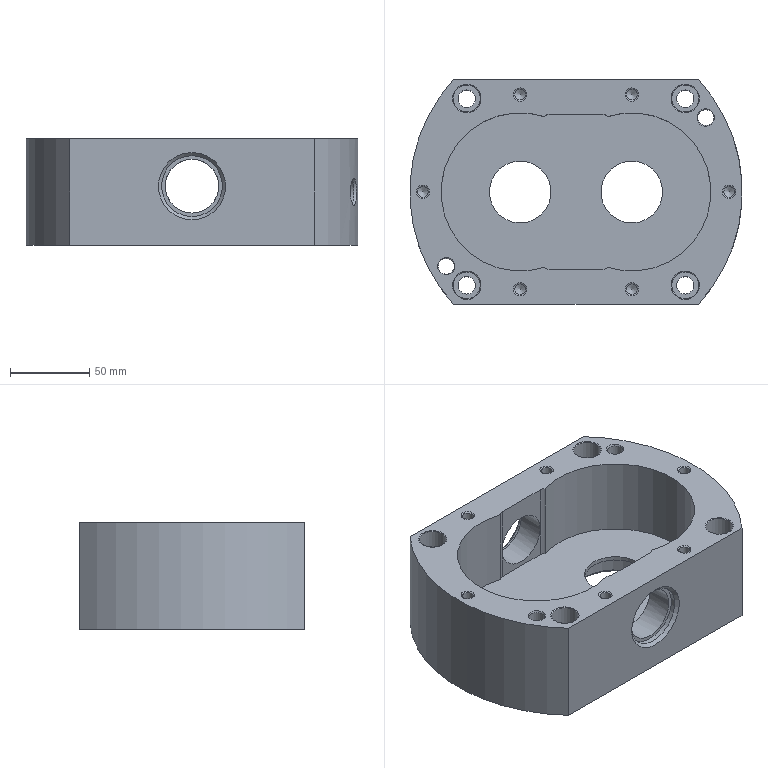NC program | NX | posted with a generic post | part box 210 x 142 x 67.4 mm
Lines 5618 to 6488 of 83330:
(ZLEVEL_PROFILE_COPY , TOOL : D6)
N11186 T06 M6
N11188 G54
N11190 G17 G0 G90 X-53.8 Y-59.497 B0. C0. S5000 M3
N11192 G43 Z30. H6
N11194 Z-0.1
N11196 G94 G1 X-54.786 Y-60.324 F1000.
N11198 G3 X-55. Y-60.784 R0.6
N11200 G1 Y-62. F1600.
N11202 G3 X-54. Y-63. R1.
N11204 G1 X-52.784
N11206 G3 X-52.324 Y-62.786 R0.6
N11208 G1 X-51.497 Y-61.8
N11210 G0 X-53.8 Y-59.497 Z-0.2
N11212 G1 X-54.786 Y-60.324 F1000.
N11214 G3 X-55. Y-60.784 R0.6
N11216 G1 Y-62. F1600.
N11218 G3 X-54. Y-63. R1.
N11220 G1 X-52.784
N11222 G3 X-52.324 Y-62.786 R0.6
N11224 G1 X-51.497 Y-61.8
N11226 G0 X-53.8 Y-59.497 Z-0.3
N11228 G1 X-54.786 Y-60.324 F1000.
N11230 G3 X-55. Y-60.784 R0.6
N11232 G1 Y-62. F1600.
N11234 G3 X-54. Y-63. R1.
N11236 G1 X-52.784
N11238 G3 X-52.324 Y-62.786 R0.6
N11240 G1 X-51.497 Y-61.8
N11242 G0 X-53.8 Y-59.497 Z-0.4
N11244 G1 X-54.786 Y-60.324 F1000.
N11246 G3 X-55. Y-60.784 R0.6
N11248 G1 Y-62. F1600.
N11250 G3 X-54. Y-63. R1.
N11252 G1 X-52.784
N11254 G3 X-52.324 Y-62.786 R0.6
N11256 G1 X-51.497 Y-61.8
N11258 G0 X-53.8 Y-59.497 Z-0.5
N11260 G1 X-54.786 Y-60.324 F1000.
N11262 G3 X-55. Y-60.784 R0.6
N11264 G1 Y-62. F1600.
N11266 G3 X-54. Y-63. R1.
N11268 G1 X-52.784
N11270 G3 X-52.324 Y-62.786 R0.6
N11272 G1 X-51.497 Y-61.8
N11274 G0 X-53.8 Y-59.497 Z-0.6
N11276 G1 X-54.786 Y-60.324 F1000.
N11278 G3 X-55. Y-60.784 R0.6
N11280 G1 Y-62. F1600.
N11282 G3 X-54. Y-63. R1.
N11284 G1 X-52.784
N11286 G3 X-52.324 Y-62.786 R0.6
N11288 G1 X-51.497 Y-61.8
N11290 G0 X-53.8 Y-59.497 Z-0.7
N11292 G1 X-54.786 Y-60.324 F1000.
N11294 G3 X-55. Y-60.784 R0.6
N11296 G1 Y-62. F1600.
N11298 G3 X-54. Y-63. R1.
N11300 G1 X-52.784
N11302 G3 X-52.324 Y-62.786 R0.6
N11304 G1 X-51.497 Y-61.8
N11306 G0 X-53.8 Y-59.497 Z-0.8
N11308 G1 X-54.786 Y-60.324 F1000.
N11310 G3 X-55. Y-60.784 R0.6
N11312 G1 Y-62. F1600.
N11314 G3 X-54. Y-63. R1.
N11316 G1 X-52.784
N11318 G3 X-52.324 Y-62.786 R0.6
N11320 G1 X-51.497 Y-61.8
N11322 G0 X-53.8 Y-59.497 Z-0.9
N11324 G1 X-54.786 Y-60.324 F1000.
N11326 G3 X-55. Y-60.784 R0.6
N11328 G1 Y-62. F1600.
N11330 G3 X-54. Y-63. R1.
N11332 G1 X-52.784
N11334 G3 X-52.324 Y-62.786 R0.6
N11336 G1 X-51.497 Y-61.8
N11338 G0 X-53.8 Y-59.497 Z-1.
N11340 G1 X-54.786 Y-60.324 F1000.
N11342 G3 X-55. Y-60.784 R0.6
N11344 G1 Y-62. F1600.
N11346 G3 X-54. Y-63. R1.
N11348 G1 X-52.784
N11350 G3 X-52.324 Y-62.786 R0.6
N11352 G1 X-51.497 Y-61.8
N11354 G0 X-53.8 Y-59.497 Z-1.1
N11356 G1 X-54.786 Y-60.324 F1000.
N11358 G3 X-55. Y-60.784 R0.6
N11360 G1 Y-62. F1600.
N11362 G3 X-54. Y-63. R1.
N11364 G1 X-52.784
N11366 G3 X-52.324 Y-62.786 R0.6
N11368 G1 X-51.497 Y-61.8
N11370 G0 X-53.8 Y-59.497 Z-1.2
N11372 G1 X-54.786 Y-60.324 F1000.
N11374 G3 X-55. Y-60.784 R0.6
N11376 G1 Y-62. F1600.
N11378 G3 X-54. Y-63. R1.
N11380 G1 X-52.784
N11382 G3 X-52.324 Y-62.786 R0.6
N11384 G1 X-51.497 Y-61.8
N11386 G0 X-53.8 Y-59.497 Z-1.3
N11388 G1 X-54.786 Y-60.324 F1000.
N11390 G3 X-55. Y-60.784 R0.6
N11392 G1 Y-62. F1600.
N11394 G3 X-54. Y-63. R1.
N11396 G1 X-52.784
N11398 G3 X-52.324 Y-62.786 R0.6
N11400 G1 X-51.497 Y-61.8
N11402 G0 X-53.8 Y-59.497 Z-1.4
N11404 G1 X-54.786 Y-60.324 F1000.
N11406 G3 X-55. Y-60.784 R0.6
N11408 G1 Y-62. F1600.
N11410 G3 X-54. Y-63. R1.
N11412 G1 X-52.784
N11414 G3 X-52.324 Y-62.786 R0.6
N11416 G1 X-51.497 Y-61.8
N11418 G0 X-53.8 Y-59.497 Z-1.5
N11420 G1 X-54.786 Y-60.324 F1000.
N11422 G3 X-55. Y-60.784 R0.6
N11424 G1 Y-62. F1600.
N11426 G3 X-54. Y-63. R1.
N11428 G1 X-52.784
N11430 G3 X-52.324 Y-62.786 R0.6
N11432 G1 X-51.497 Y-61.8
N11434 G0 X-53.8 Y-59.497 Z-1.6
N11436 G1 X-54.786 Y-60.324 F1000.
N11438 G3 X-55. Y-60.784 R0.6
N11440 G1 Y-62. F1600.
N11442 G3 X-54. Y-63. R1.
N11444 G1 X-52.784
N11446 G3 X-52.324 Y-62.786 R0.6
N11448 G1 X-51.497 Y-61.8
N11450 G0 X-53.8 Y-59.497 Z-1.7
N11452 G1 X-54.786 Y-60.324 F1000.
N11454 G3 X-55. Y-60.784 R0.6
N11456 G1 Y-62. F1600.
N11458 G3 X-54. Y-63. R1.
N11460 G1 X-52.784
N11462 G3 X-52.324 Y-62.786 R0.6
N11464 G1 X-51.497 Y-61.8
N11466 G0 X-53.8 Y-59.497 Z-1.8
N11468 G1 X-54.786 Y-60.324 F1000.
N11470 G3 X-55. Y-60.784 R0.6
N11472 G1 Y-62. F1600.
N11474 G3 X-54. Y-63. R1.
N11476 G1 X-52.784
N11478 G3 X-52.324 Y-62.786 R0.6
N11480 G1 X-51.497 Y-61.8
N11482 G0 X-53.8 Y-59.497 Z-1.9
N11484 G1 X-54.786 Y-60.324 F1000.
N11486 G3 X-55. Y-60.784 R0.6
N11488 G1 Y-62. F1600.
N11490 G3 X-54. Y-63. R1.
N11492 G1 X-52.784
N11494 G3 X-52.324 Y-62.786 R0.6
N11496 G1 X-51.497 Y-61.8
N11498 G0 X-53.8 Y-59.497 Z-2.
N11500 G1 X-54.786 Y-60.324 F1000.
N11502 G3 X-55. Y-60.784 R0.6
N11504 G1 Y-62. F1600.
N11506 G3 X-54. Y-63. R1.
N11508 G1 X-52.784
N11510 G3 X-52.324 Y-62.786 R0.6
N11512 G1 X-51.497 Y-61.8
N11514 G0 X-53.8 Y-59.497 Z-2.1
N11516 G1 X-54.786 Y-60.324 F1000.
N11518 G3 X-55. Y-60.784 R0.6
N11520 G1 Y-62. F1600.
N11522 G3 X-54. Y-63. R1.
N11524 G1 X-52.784
N11526 G3 X-52.324 Y-62.786 R0.6
N11528 G1 X-51.497 Y-61.8
N11530 G0 X-53.8 Y-59.497 Z-2.2
N11532 G1 X-54.786 Y-60.324 F1000.
N11534 G3 X-55. Y-60.784 R0.6
N11536 G1 Y-62. F1600.
N11538 G3 X-54. Y-63. R1.
N11540 G1 X-52.784
N11542 G3 X-52.324 Y-62.786 R0.6
N11544 G1 X-51.497 Y-61.8
N11546 G0 X-53.8 Y-59.497 Z-2.3
N11548 G1 X-54.786 Y-60.324 F1000.
N11550 G3 X-55. Y-60.784 R0.6
N11552 G1 Y-62. F1600.
N11554 G3 X-54. Y-63. R1.
N11556 G1 X-52.784
N11558 G3 X-52.324 Y-62.786 R0.6
N11560 G1 X-51.497 Y-61.8
N11562 G0 X-53.8 Y-59.497 Z-2.4
N11564 G1 X-54.786 Y-60.324 F1000.
N11566 G3 X-55. Y-60.784 R0.6
N11568 G1 Y-62. F1600.
N11570 G3 X-54. Y-63. R1.
N11572 G1 X-52.784
N11574 G3 X-52.324 Y-62.786 R0.6
N11576 G1 X-51.497 Y-61.8
N11578 G0 X-53.8 Y-59.497 Z-2.5
N11580 G1 X-54.786 Y-60.324 F1000.
N11582 G3 X-55. Y-60.784 R0.6
N11584 G1 Y-62. F1600.
N11586 G3 X-54. Y-63. R1.
N11588 G1 X-52.784
N11590 G3 X-52.324 Y-62.786 R0.6
N11592 G1 X-51.497 Y-61.8
N11594 G0 X-53.8 Y-59.497 Z-2.6
N11596 G1 X-54.786 Y-60.324 F1000.
N11598 G3 X-55. Y-60.784 R0.6
N11600 G1 Y-62. F1600.
N11602 G3 X-54. Y-63. R1.
N11604 G1 X-52.784
N11606 G3 X-52.324 Y-62.786 R0.6
N11608 G1 X-51.497 Y-61.8
N11610 G0 X-53.8 Y-59.497 Z-2.7
N11612 G1 X-54.786 Y-60.324 F1000.
N11614 G3 X-55. Y-60.784 R0.6
N11616 G1 Y-62. F1600.
N11618 G3 X-54. Y-63. R1.
N11620 G1 X-52.784
N11622 G3 X-52.324 Y-62.786 R0.6
N11624 G1 X-51.497 Y-61.8
N11626 G0 X-53.8 Y-59.497 Z-2.8
N11628 G1 X-54.786 Y-60.324 F1000.
N11630 G3 X-55. Y-60.784 R0.6
N11632 G1 Y-62. F1600.
N11634 G3 X-54. Y-63. R1.
N11636 G1 X-52.784
N11638 G3 X-52.324 Y-62.786 R0.6
N11640 G1 X-51.497 Y-61.8
N11642 G0 X-53.8 Y-59.497 Z-2.9
N11644 G1 X-54.786 Y-60.324 F1000.
N11646 G3 X-55. Y-60.784 R0.6
N11648 G1 Y-62. F1600.
N11650 G3 X-54. Y-63. R1.
N11652 G1 X-52.784
N11654 G3 X-52.324 Y-62.786 R0.6
N11656 G1 X-51.497 Y-61.8
N11658 G0 X-53.8 Y-59.497 Z-3.
N11660 G1 X-54.786 Y-60.324 F1000.
N11662 G3 X-55. Y-60.784 R0.6
N11664 G1 Y-62. F1600.
N11666 G3 X-54. Y-63. R1.
N11668 G1 X-52.784
N11670 G3 X-52.324 Y-62.786 R0.6
N11672 G1 X-51.497 Y-61.8
N11674 G0 X-53.8 Y-59.497 Z-3.1
N11676 G1 X-54.786 Y-60.324 F1000.
N11678 G3 X-55. Y-60.784 R0.6
N11680 G1 Y-62. F1600.
N11682 G3 X-54. Y-63. R1.
N11684 G1 X-52.784
N11686 G3 X-52.324 Y-62.786 R0.6
N11688 G1 X-51.497 Y-61.8
N11690 G0 X-53.8 Y-59.497 Z-3.2
N11692 G1 X-54.786 Y-60.324 F1000.
N11694 G3 X-55. Y-60.784 R0.6
N11696 G1 Y-62. F1600.
N11698 G3 X-54. Y-63. R1.
N11700 G1 X-52.784
N11702 G3 X-52.324 Y-62.786 R0.6
N11704 G1 X-51.497 Y-61.8
N11706 G0 X-53.8 Y-59.497 Z-3.3
N11708 G1 X-54.786 Y-60.324 F1000.
N11710 G3 X-55. Y-60.784 R0.6
N11712 G1 Y-62. F1600.
N11714 G3 X-54. Y-63. R1.
N11716 G1 X-52.784
N11718 G3 X-52.324 Y-62.786 R0.6
N11720 G1 X-51.497 Y-61.8
N11722 G0 X-53.8 Y-59.497 Z-3.4
N11724 G1 X-54.786 Y-60.324 F1000.
N11726 G3 X-55. Y-60.784 R0.6
N11728 G1 Y-62. F1600.
N11730 G3 X-54. Y-63. R1.
N11732 G1 X-52.784
N11734 G3 X-52.324 Y-62.786 R0.6
N11736 G1 X-51.497 Y-61.8
N11738 G0 X-53.8 Y-59.497 Z-3.5
N11740 G1 X-54.786 Y-60.324 F1000.
N11742 G3 X-55. Y-60.784 R0.6
N11744 G1 Y-62. F1600.
N11746 G3 X-54. Y-63. R1.
N11748 G1 X-52.784
N11750 G3 X-52.324 Y-62.786 R0.6
N11752 G1 X-51.497 Y-61.8
N11754 G0 X-53.8 Y-59.497 Z-3.6
N11756 G1 X-54.786 Y-60.324 F1000.
N11758 G3 X-55. Y-60.784 R0.6
N11760 G1 Y-62. F1600.
N11762 G3 X-54. Y-63. R1.
N11764 G1 X-52.784
N11766 G3 X-52.324 Y-62.786 R0.6
N11768 G1 X-51.497 Y-61.8
N11770 G0 X-53.8 Y-59.497 Z-3.7
N11772 G1 X-54.786 Y-60.324 F1000.
N11774 G3 X-55. Y-60.784 R0.6
N11776 G1 Y-62. F1600.
N11778 G3 X-54. Y-63. R1.
N11780 G1 X-52.784
N11782 G3 X-52.324 Y-62.786 R0.6
N11784 G1 X-51.497 Y-61.8
N11786 G0 X-53.8 Y-59.497 Z-3.8
N11788 G1 X-54.786 Y-60.324 F1000.
N11790 G3 X-55. Y-60.784 R0.6
N11792 G1 Y-62. F1600.
N11794 G3 X-54. Y-63. R1.
N11796 G1 X-52.784
N11798 G3 X-52.324 Y-62.786 R0.6
N11800 G1 X-51.497 Y-61.8
N11802 G0 X-53.8 Y-59.497 Z-3.9
N11804 G1 X-54.786 Y-60.324 F1000.
N11806 G3 X-55. Y-60.784 R0.6
N11808 G1 Y-62. F1600.
N11810 G3 X-54. Y-63. R1.
N11812 G1 X-52.784
N11814 G3 X-52.324 Y-62.786 R0.6
N11816 G1 X-51.497 Y-61.8
N11818 G0 X-53.8 Y-59.497 Z-4.
N11820 G1 X-54.786 Y-60.324 F1000.
N11822 G3 X-55. Y-60.784 R0.6
N11824 G1 Y-62. F1600.
N11826 G3 X-54. Y-63. R1.
N11828 G1 X-52.784
N11830 G3 X-52.324 Y-62.786 R0.6
N11832 G1 X-51.497 Y-61.8
N11834 G0 X-53.8 Y-59.497 Z-4.1
N11836 G1 X-54.786 Y-60.324 F1000.
N11838 G3 X-55. Y-60.784 R0.6
N11840 G1 Y-62. F1600.
N11842 G3 X-54. Y-63. R1.
N11844 G1 X-52.784
N11846 G3 X-52.324 Y-62.786 R0.6
N11848 G1 X-51.497 Y-61.8
N11850 G0 X-53.8 Y-59.497 Z-4.2
N11852 G1 X-54.786 Y-60.324 F1000.
N11854 G3 X-55. Y-60.784 R0.6
N11856 G1 Y-62. F1600.
N11858 G3 X-54. Y-63. R1.
N11860 G1 X-52.784
N11862 G3 X-52.324 Y-62.786 R0.6
N11864 G1 X-51.497 Y-61.8
N11866 G0 X-53.8 Y-59.497 Z-4.3
N11868 G1 X-54.786 Y-60.324 F1000.
N11870 G3 X-55. Y-60.784 R0.6
N11872 G1 Y-62. F1600.
N11874 G3 X-54. Y-63. R1.
N11876 G1 X-52.784
N11878 G3 X-52.324 Y-62.786 R0.6
N11880 G1 X-51.497 Y-61.8
N11882 G0 X-53.8 Y-59.497 Z-4.4
N11884 G1 X-54.786 Y-60.324 F1000.
N11886 G3 X-55. Y-60.784 R0.6
N11888 G1 Y-62. F1600.
N11890 G3 X-54. Y-63. R1.
N11892 G1 X-52.784
N11894 G3 X-52.324 Y-62.786 R0.6
N11896 G1 X-51.497 Y-61.8
N11898 G0 X-53.8 Y-59.497 Z-4.5
N11900 G1 X-54.786 Y-60.324 F1000.
N11902 G3 X-55. Y-60.784 R0.6
N11904 G1 Y-62. F1600.
N11906 G3 X-54. Y-63. R1.
N11908 G1 X-52.784
N11910 G3 X-52.324 Y-62.786 R0.6
N11912 G1 X-51.497 Y-61.8
N11914 G0 X-53.8 Y-59.497 Z-4.6
N11916 G1 X-54.786 Y-60.324 F1000.
N11918 G3 X-55. Y-60.784 R0.6
N11920 G1 Y-62. F1600.
N11922 G3 X-54. Y-63. R1.
N11924 G1 X-52.784
N11926 G3 X-52.324 Y-62.786 R0.6
N11928 G1 X-51.497 Y-61.8
N11930 G0 X-53.8 Y-59.497 Z-4.7
N11932 G1 X-54.786 Y-60.324 F1000.
N11934 G3 X-55. Y-60.784 R0.6
N11936 G1 Y-62. F1600.
N11938 G3 X-54. Y-63. R1.
N11940 G1 X-52.784
N11942 G3 X-52.324 Y-62.786 R0.6
N11944 G1 X-51.497 Y-61.8
N11946 G0 X-53.8 Y-59.497 Z-4.8
N11948 G1 X-54.786 Y-60.324 F1000.
N11950 G3 X-55. Y-60.784 R0.6
N11952 G1 Y-62. F1600.
N11954 G3 X-54. Y-63. R1.
N11956 G1 X-52.784
N11958 G3 X-52.324 Y-62.786 R0.6
N11960 G1 X-51.497 Y-61.8
N11962 G0 X-53.8 Y-59.497 Z-4.9
N11964 G1 X-54.786 Y-60.324 F1000.
N11966 G3 X-55. Y-60.784 R0.6
N11968 G1 Y-62. F1600.
N11970 G3 X-54. Y-63. R1.
N11972 G1 X-52.784
N11974 G3 X-52.324 Y-62.786 R0.6
N11976 G1 X-51.497 Y-61.8
N11978 G0 X-53.8 Y-59.497 Z-5.
N11980 G1 X-54.786 Y-60.324 F1000.
N11982 G3 X-55. Y-60.784 R0.6
N11984 G1 Y-62. F1600.
N11986 G3 X-54. Y-63. R1.
N11988 G1 X-52.784
N11990 G3 X-52.324 Y-62.786 R0.6
N11992 G1 X-51.497 Y-61.8
N11994 G0 X-53.8 Y-59.497 Z-5.1
N11996 G1 X-54.786 Y-60.324 F1000.
N11998 G3 X-55. Y-60.784 R0.6
N12000 G1 Y-62. F1600.
N12002 G3 X-54. Y-63. R1.
N12004 G1 X-52.784
N12006 G3 X-52.324 Y-62.786 R0.6
N12008 G1 X-51.497 Y-61.8
N12010 G0 X-53.8 Y-59.497 Z-5.2
N12012 G1 X-54.786 Y-60.324 F1000.
N12014 G3 X-55. Y-60.784 R0.6
N12016 G1 Y-62. F1600.
N12018 G3 X-54. Y-63. R1.
N12020 G1 X-52.784
N12022 G3 X-52.324 Y-62.786 R0.6
N12024 G1 X-51.497 Y-61.8
N12026 G0 X-53.8 Y-59.497 Z-5.3
N12028 G1 X-54.786 Y-60.324 F1000.
N12030 G3 X-55. Y-60.784 R0.6
N12032 G1 Y-62. F1600.
N12034 G3 X-54. Y-63. R1.
N12036 G1 X-52.784
N12038 G3 X-52.324 Y-62.786 R0.6
N12040 G1 X-51.497 Y-61.8
N12042 G0 X-53.8 Y-59.497 Z-5.4
N12044 G1 X-54.786 Y-60.324 F1000.
N12046 G3 X-55. Y-60.784 R0.6
N12048 G1 Y-62. F1600.
N12050 G3 X-54. Y-63. R1.
N12052 G1 X-52.784
N12054 G3 X-52.324 Y-62.786 R0.6
N12056 G1 X-51.497 Y-61.8
N12058 G0 X-53.8 Y-59.497 Z-5.5
N12060 G1 X-54.786 Y-60.324 F1000.
N12062 G3 X-55. Y-60.784 R0.6
N12064 G1 Y-62. F1600.
N12066 G3 X-54. Y-63. R1.
N12068 G1 X-52.784
N12070 G3 X-52.324 Y-62.786 R0.6
N12072 G1 X-51.497 Y-61.8
N12074 G0 X-53.8 Y-59.497 Z-5.6
N12076 G1 X-54.786 Y-60.324 F1000.
N12078 G3 X-55. Y-60.784 R0.6
N12080 G1 Y-62. F1600.
N12082 G3 X-54. Y-63. R1.
N12084 G1 X-52.784
N12086 G3 X-52.324 Y-62.786 R0.6
N12088 G1 X-51.497 Y-61.8
N12090 G0 X-53.8 Y-59.497 Z-5.7
N12092 G1 X-54.786 Y-60.324 F1000.
N12094 G3 X-55. Y-60.784 R0.6
N12096 G1 Y-62. F1600.
N12098 G3 X-54. Y-63. R1.
N12100 G1 X-52.784
N12102 G3 X-52.324 Y-62.786 R0.6
N12104 G1 X-51.497 Y-61.8
N12106 G0 X-53.8 Y-59.497 Z-5.8
N12108 G1 X-54.786 Y-60.324 F1000.
N12110 G3 X-55. Y-60.784 R0.6
N12112 G1 Y-62. F1600.
N12114 G3 X-54. Y-63. R1.
N12116 G1 X-52.784
N12118 G3 X-52.324 Y-62.786 R0.6
N12120 G1 X-51.497 Y-61.8
N12122 G0 X-53.8 Y-59.497 Z-5.9
N12124 G1 X-54.786 Y-60.324 F1000.
N12126 G3 X-55. Y-60.784 R0.6
N12128 G1 Y-62. F1600.
N12130 G3 X-54. Y-63. R1.
N12132 G1 X-52.784
N12134 G3 X-52.324 Y-62.786 R0.6
N12136 G1 X-51.497 Y-61.8
N12138 G0 X-53.8 Y-59.497 Z-6.
N12140 G1 X-54.786 Y-60.324 F1000.
N12142 G3 X-55. Y-60.784 R0.6
N12144 G1 Y-62. F1600.
N12146 G3 X-54. Y-63. R1.
N12148 G1 X-52.784
N12150 G3 X-52.324 Y-62.786 R0.6
N12152 G1 X-51.497 Y-61.8
N12154 G0 X-53.8 Y-59.497 Z-6.1
N12156 G1 X-54.786 Y-60.324 F1000.
N12158 G3 X-55. Y-60.784 R0.6
N12160 G1 Y-62. F1600.
N12162 G3 X-54. Y-63. R1.
N12164 G1 X-52.784
N12166 G3 X-52.324 Y-62.786 R0.6
N12168 G1 X-51.497 Y-61.8
N12170 G0 X-53.8 Y-59.497 Z-6.2
N12172 G1 X-54.786 Y-60.324 F1000.
N12174 G3 X-55. Y-60.784 R0.6
N12176 G1 Y-62. F1600.
N12178 G3 X-54. Y-63. R1.
N12180 G1 X-52.784
N12182 G3 X-52.324 Y-62.786 R0.6
N12184 G1 X-51.497 Y-61.8
N12186 G0 X-53.8 Y-59.497 Z-6.3
N12188 G1 X-54.786 Y-60.324 F1000.
N12190 G3 X-55. Y-60.784 R0.6
N12192 G1 Y-62. F1600.
N12194 G3 X-54. Y-63. R1.
N12196 G1 X-52.784
N12198 G3 X-52.324 Y-62.786 R0.6
N12200 G1 X-51.497 Y-61.8
N12202 G0 X-53.8 Y-59.497 Z-6.4
N12204 G1 X-54.786 Y-60.324 F1000.
N12206 G3 X-55. Y-60.784 R0.6
N12208 G1 Y-62. F1600.
N12210 G3 X-54. Y-63. R1.
N12212 G1 X-52.784
N12214 G3 X-52.324 Y-62.786 R0.6
N12216 G1 X-51.497 Y-61.8
N12218 G0 X-53.8 Y-59.497 Z-6.5
N12220 G1 X-54.786 Y-60.324 F1000.
N12222 G3 X-55. Y-60.784 R0.6
N12224 G1 Y-62. F1600.
N12226 G3 X-54. Y-63. R1.
N12228 G1 X-52.784
N12230 G3 X-52.324 Y-62.786 R0.6
N12232 G1 X-51.497 Y-61.8
N12234 G0 X-53.8 Y-59.497 Z-6.6
N12236 G1 X-54.786 Y-60.324 F1000.
N12238 G3 X-55. Y-60.784 R0.6
N12240 G1 Y-62. F1600.
N12242 G3 X-54. Y-63. R1.
N12244 G1 X-52.784
N12246 G3 X-52.324 Y-62.786 R0.6
N12248 G1 X-51.497 Y-61.8
N12250 G0 X-53.8 Y-59.497 Z-6.7
N12252 G1 X-54.786 Y-60.324 F1000.
N12254 G3 X-55. Y-60.784 R0.6
N12256 G1 Y-62. F1600.
N12258 G3 X-54. Y-63. R1.
N12260 G1 X-52.784
N12262 G3 X-52.324 Y-62.786 R0.6
N12264 G1 X-51.497 Y-61.8
N12266 G0 X-53.8 Y-59.497 Z-6.8
N12268 G1 X-54.786 Y-60.324 F1000.
N12270 G3 X-55. Y-60.784 R0.6
N12272 G1 Y-62. F1600.
N12274 G3 X-54. Y-63. R1.
N12276 G1 X-52.784
N12278 G3 X-52.324 Y-62.786 R0.6
N12280 G1 X-51.497 Y-61.8
N12282 G0 X-53.8 Y-59.497 Z-6.9
N12284 G1 X-54.786 Y-60.324 F1000.
N12286 G3 X-55. Y-60.784 R0.6
N12288 G1 Y-62. F1600.
N12290 G3 X-54. Y-63. R1.
N12292 G1 X-52.784
N12294 G3 X-52.324 Y-62.786 R0.6
N12296 G1 X-51.497 Y-61.8
N12298 G0 X-53.8 Y-59.497 Z-7.
N12300 G1 X-54.786 Y-60.324 F1000.
N12302 G3 X-55. Y-60.784 R0.6
N12304 G1 Y-62. F1600.
N12306 G3 X-54. Y-63. R1.
N12308 G1 X-52.784
N12310 G3 X-52.324 Y-62.786 R0.6
N12312 G1 X-51.497 Y-61.8
N12314 G0 Z30.
N12316 X51.497
N12318 Z-0.1
N12320 G1 X52.324 Y-62.786 F1000.
N12322 G3 X52.784 Y-63. R0.6
N12324 G1 X54. F1600.
N12326 G3 X55. Y-62. R1.
N12328 G1 Y-60.784
N12330 G3 X54.786 Y-60.324 R0.6
N12332 G1 X53.8 Y-59.497
N12334 G0 X51.497 Y-61.8 Z-0.2
N12336 G1 X52.324 Y-62.786 F1000.
N12338 G3 X52.784 Y-63. R0.6
N12340 G1 X54. F1600.
N12342 G3 X55. Y-62. R1.
N12344 G1 Y-60.784
N12346 G3 X54.786 Y-60.324 R0.6
N12348 G1 X53.8 Y-59.497
N12350 G0 X51.497 Y-61.8 Z-0.3
N12352 G1 X52.324 Y-62.786 F1000.
N12354 G3 X52.784 Y-63. R0.6
N12356 G1 X54. F1600.
N12358 G3 X55. Y-62. R1.
N12360 G1 Y-60.784
N12362 G3 X54.786 Y-60.324 R0.6
N12364 G1 X53.8 Y-59.497
N12366 G0 X51.497 Y-61.8 Z-0.4
N12368 G1 X52.324 Y-62.786 F1000.
N12370 G3 X52.784 Y-63. R0.6
N12372 G1 X54. F1600.
N12374 G3 X55. Y-62. R1.
N12376 G1 Y-60.784
N12378 G3 X54.786 Y-60.324 R0.6
N12380 G1 X53.8 Y-59.497
N12382 G0 X51.497 Y-61.8 Z-0.5
N12384 G1 X52.324 Y-62.786 F1000.
N12386 G3 X52.784 Y-63. R0.6
N12388 G1 X54. F1600.
N12390 G3 X55. Y-62. R1.
N12392 G1 Y-60.784
N12394 G3 X54.786 Y-60.324 R0.6
N12396 G1 X53.8 Y-59.497
N12398 G0 X51.497 Y-61.8 Z-0.6
N12400 G1 X52.324 Y-62.786 F1000.
N12402 G3 X52.784 Y-63. R0.6
N12404 G1 X54. F1600.
N12406 G3 X55. Y-62. R1.
N12408 G1 Y-60.784
N12410 G3 X54.786 Y-60.324 R0.6
N12412 G1 X53.8 Y-59.497
N12414 G0 X51.497 Y-61.8 Z-0.7
N12416 G1 X52.324 Y-62.786 F1000.
N12418 G3 X52.784 Y-63. R0.6
N12420 G1 X54. F1600.
N12422 G3 X55. Y-62. R1.
N12424 G1 Y-60.784
N12426 G3 X54.786 Y-60.324 R0.6
N12428 G1 X53.8 Y-59.497
N12430 G0 X51.497 Y-61.8 Z-0.8
N12432 G1 X52.324 Y-62.786 F1000.
N12434 G3 X52.784 Y-63. R0.6
N12436 G1 X54. F1600.
N12438 G3 X55. Y-62. R1.
N12440 G1 Y-60.784
N12442 G3 X54.786 Y-60.324 R0.6
N12444 G1 X53.8 Y-59.497
N12446 G0 X51.497 Y-61.8 Z-0.9
N12448 G1 X52.324 Y-62.786 F1000.
N12450 G3 X52.784 Y-63. R0.6
N12452 G1 X54. F1600.
N12454 G3 X55. Y-62. R1.
N12456 G1 Y-60.784
N12458 G3 X54.786 Y-60.324 R0.6
N12460 G1 X53.8 Y-59.497
N12462 G0 X51.497 Y-61.8 Z-1.
N12464 G1 X52.324 Y-62.786 F1000.
N12466 G3 X52.784 Y-63. R0.6
N12468 G1 X54. F1600.
N12470 G3 X55. Y-62. R1.
N12472 G1 Y-60.784
N12474 G3 X54.786 Y-60.324 R0.6
N12476 G1 X53.8 Y-59.497
N12478 G0 X51.497 Y-61.8 Z-1.1
N12480 G1 X52.324 Y-62.786 F1000.
N12482 G3 X52.784 Y-63. R0.6
N12484 G1 X54. F1600.
N12486 G3 X55. Y-62. R1.
N12488 G1 Y-60.784
N12490 G3 X54.786 Y-60.324 R0.6
N12492 G1 X53.8 Y-59.497
N12494 G0 X51.497 Y-61.8 Z-1.2
N12496 G1 X52.324 Y-62.786 F1000.
N12498 G3 X52.784 Y-63. R0.6
N12500 G1 X54. F1600.
N12502 G3 X55. Y-62. R1.
N12504 G1 Y-60.784
N12506 G3 X54.786 Y-60.324 R0.6
N12508 G1 X53.8 Y-59.497
N12510 G0 X51.497 Y-61.8 Z-1.3
N12512 G1 X52.324 Y-62.786 F1000.
N12514 G3 X52.784 Y-63. R0.6
N12516 G1 X54. F1600.
N12518 G3 X55. Y-62. R1.
N12520 G1 Y-60.784
N12522 G3 X54.786 Y-60.324 R0.6
N12524 G1 X53.8 Y-59.497
N12526 G0 X51.497 Y-61.8 Z-1.4
N12528 G1 X52.324 Y-62.786 F1000.
N12530 G3 X52.784 Y-63. R0.6
N12532 G1 X54. F1600.
N12534 G3 X55. Y-62. R1.
N12536 G1 Y-60.784
N12538 G3 X54.786 Y-60.324 R0.6
N12540 G1 X53.8 Y-59.497
N12542 G0 X51.497 Y-61.8 Z-1.5
N12544 G1 X52.324 Y-62.786 F1000.
N12546 G3 X52.784 Y-63. R0.6
N12548 G1 X54. F1600.
N12550 G3 X55. Y-62. R1.
N12552 G1 Y-60.784
N12554 G3 X54.786 Y-60.324 R0.6
N12556 G1 X53.8 Y-59.497
N12558 G0 X51.497 Y-61.8 Z-1.6
N12560 G1 X52.324 Y-62.786 F1000.
N12562 G3 X52.784 Y-63. R0.6
N12564 G1 X54. F1600.
N12566 G3 X55. Y-62. R1.
N12568 G1 Y-60.784
N12570 G3 X54.786 Y-60.324 R0.6
N12572 G1 X53.8 Y-59.497
N12574 G0 X51.497 Y-61.8 Z-1.7
N12576 G1 X52.324 Y-62.786 F1000.
N12578 G3 X52.784 Y-63. R0.6
N12580 G1 X54. F1600.
N12582 G3 X55. Y-62. R1.
N12584 G1 Y-60.784
N12586 G3 X54.786 Y-60.324 R0.6
N12588 G1 X53.8 Y-59.497
N12590 G0 X51.497 Y-61.8 Z-1.8
N12592 G1 X52.324 Y-62.786 F1000.
N12594 G3 X52.784 Y-63. R0.6
N12596 G1 X54. F1600.
N12598 G3 X55. Y-62. R1.
N12600 G1 Y-60.784
N12602 G3 X54.786 Y-60.324 R0.6
N12604 G1 X53.8 Y-59.497
N12606 G0 X51.497 Y-61.8 Z-1.9
N12608 G1 X52.324 Y-62.786 F1000.
N12610 G3 X52.784 Y-63. R0.6
N12612 G1 X54. F1600.
N12614 G3 X55. Y-62. R1.
N12616 G1 Y-60.784
N12618 G3 X54.786 Y-60.324 R0.6
N12620 G1 X53.8 Y-59.497
N12622 G0 X51.497 Y-61.8 Z-2.
N12624 G1 X52.324 Y-62.786 F1000.
N12626 G3 X52.784 Y-63. R0.6
N12628 G1 X54. F1600.
N12630 G3 X55. Y-62. R1.
N12632 G1 Y-60.784
N12634 G3 X54.786 Y-60.324 R0.6
N12636 G1 X53.8 Y-59.497
N12638 G0 X51.497 Y-61.8 Z-2.1
N12640 G1 X52.324 Y-62.786 F1000.
N12642 G3 X52.784 Y-63. R0.6
N12644 G1 X54. F1600.
N12646 G3 X55. Y-62. R1.
N12648 G1 Y-60.784
N12650 G3 X54.786 Y-60.324 R0.6
N12652 G1 X53.8 Y-59.497
N12654 G0 X51.497 Y-61.8 Z-2.2
N12656 G1 X52.324 Y-62.786 F1000.
N12658 G3 X52.784 Y-63. R0.6
N12660 G1 X54. F1600.
N12662 G3 X55. Y-62. R1.
N12664 G1 Y-60.784
N12666 G3 X54.786 Y-60.324 R0.6
N12668 G1 X53.8 Y-59.497
N12670 G0 X51.497 Y-61.8 Z-2.3
N12672 G1 X52.324 Y-62.786 F1000.
N12674 G3 X52.784 Y-63. R0.6
N12676 G1 X54. F1600.
N12678 G3 X55. Y-62. R1.
N12680 G1 Y-60.784
N12682 G3 X54.786 Y-60.324 R0.6
N12684 G1 X53.8 Y-59.497
N12686 G0 X51.497 Y-61.8 Z-2.4
N12688 G1 X52.324 Y-62.786 F1000.
N12690 G3 X52.784 Y-63. R0.6
N12692 G1 X54. F1600.
N12694 G3 X55. Y-62. R1.
N12696 G1 Y-60.784
N12698 G3 X54.786 Y-60.324 R0.6
N12700 G1 X53.8 Y-59.497
N12702 G0 X51.497 Y-61.8 Z-2.5
N12704 G1 X52.324 Y-62.786 F1000.
N12706 G3 X52.784 Y-63. R0.6
N12708 G1 X54. F1600.
N12710 G3 X55. Y-62. R1.
N12712 G1 Y-60.784
N12714 G3 X54.786 Y-60.324 R0.6
N12716 G1 X53.8 Y-59.497
N12718 G0 X51.497 Y-61.8 Z-2.6
N12720 G1 X52.324 Y-62.786 F1000.
N12722 G3 X52.784 Y-63. R0.6
N12724 G1 X54. F1600.
N12726 G3 X55. Y-62. R1.
N12728 G1 Y-60.784
N12730 G3 X54.786 Y-60.324 R0.6
N12732 G1 X53.8 Y-59.497
N12734 G0 X51.497 Y-61.8 Z-2.7
N12736 G1 X52.324 Y-62.786 F1000.
N12738 G3 X52.784 Y-63. R0.6
N12740 G1 X54. F1600.
N12742 G3 X55. Y-62. R1.
N12744 G1 Y-60.784
N12746 G3 X54.786 Y-60.324 R0.6
N12748 G1 X53.8 Y-59.497
N12750 G0 X51.497 Y-61.8 Z-2.8
N12752 G1 X52.324 Y-62.786 F1000.
N12754 G3 X52.784 Y-63. R0.6
N12756 G1 X54. F1600.
N12758 G3 X55. Y-62. R1.
N12760 G1 Y-60.784
N12762 G3 X54.786 Y-60.324 R0.6
N12764 G1 X53.8 Y-59.497
N12766 G0 X51.497 Y-61.8 Z-2.9
N12768 G1 X52.324 Y-62.786 F1000.
N12770 G3 X52.784 Y-63. R0.6
N12772 G1 X54. F1600.
N12774 G3 X55. Y-62. R1.
N12776 G1 Y-60.784
N12778 G3 X54.786 Y-60.324 R0.6
N12780 G1 X53.8 Y-59.497
N12782 G0 X51.497 Y-61.8 Z-3.
N12784 G1 X52.324 Y-62.786 F1000.
N12786 G3 X52.784 Y-63. R0.6
N12788 G1 X54. F1600.
N12790 G3 X55. Y-62. R1.
N12792 G1 Y-60.784
N12794 G3 X54.786 Y-60.324 R0.6
N12796 G1 X53.8 Y-59.497
N12798 G0 X51.497 Y-61.8 Z-3.1
N12800 G1 X52.324 Y-62.786 F1000.
N12802 G3 X52.784 Y-63. R0.6
N12804 G1 X54. F1600.
N12806 G3 X55. Y-62. R1.
N12808 G1 Y-60.784
N12810 G3 X54.786 Y-60.324 R0.6
N12812 G1 X53.8 Y-59.497
N12814 G0 X51.497 Y-61.8 Z-3.2
N12816 G1 X52.324 Y-62.786 F1000.
N12818 G3 X52.784 Y-63. R0.6
N12820 G1 X54. F1600.
N12822 G3 X55. Y-62. R1.
N12824 G1 Y-60.784
N12826 G3 X54.786 Y-60.324 R0.6
N12828 G1 X53.8 Y-59.497
N12830 G0 X51.497 Y-61.8 Z-3.3
N12832 G1 X52.324 Y-62.786 F1000.
N12834 G3 X52.784 Y-63. R0.6
N12836 G1 X54. F1600.
N12838 G3 X55. Y-62. R1.
N12840 G1 Y-60.784
N12842 G3 X54.786 Y-60.324 R0.6
N12844 G1 X53.8 Y-59.497
N12846 G0 X51.497 Y-61.8 Z-3.4
N12848 G1 X52.324 Y-62.786 F1000.
N12850 G3 X52.784 Y-63. R0.6
N12852 G1 X54. F1600.
N12854 G3 X55. Y-62. R1.
N12856 G1 Y-60.784
N12858 G3 X54.786 Y-60.324 R0.6
N12860 G1 X53.8 Y-59.497
N12862 G0 X51.497 Y-61.8 Z-3.5
N12864 G1 X52.324 Y-62.786 F1000.
N12866 G3 X52.784 Y-63. R0.6
N12868 G1 X54. F1600.
N12870 G3 X55. Y-62. R1.
N12872 G1 Y-60.784
N12874 G3 X54.786 Y-60.324 R0.6
N12876 G1 X53.8 Y-59.497
N12878 G0 X51.497 Y-61.8 Z-3.6
N12880 G1 X52.324 Y-62.786 F1000.
N12882 G3 X52.784 Y-63. R0.6
N12884 G1 X54. F1600.
N12886 G3 X55. Y-62. R1.
N12888 G1 Y-60.784
N12890 G3 X54.786 Y-60.324 R0.6
N12892 G1 X53.8 Y-59.497
N12894 G0 X51.497 Y-61.8 Z-3.7
N12896 G1 X52.324 Y-62.786 F1000.
N12898 G3 X52.784 Y-63. R0.6
N12900 G1 X54. F1600.
N12902 G3 X55. Y-62. R1.
N12904 G1 Y-60.784
N12906 G3 X54.786 Y-60.324 R0.6
N12908 G1 X53.8 Y-59.497
N12910 G0 X51.497 Y-61.8 Z-3.8
N12912 G1 X52.324 Y-62.786 F1000.
N12914 G3 X52.784 Y-63. R0.6
N12916 G1 X54. F1600.
N12918 G3 X55. Y-62. R1.
N12920 G1 Y-60.784